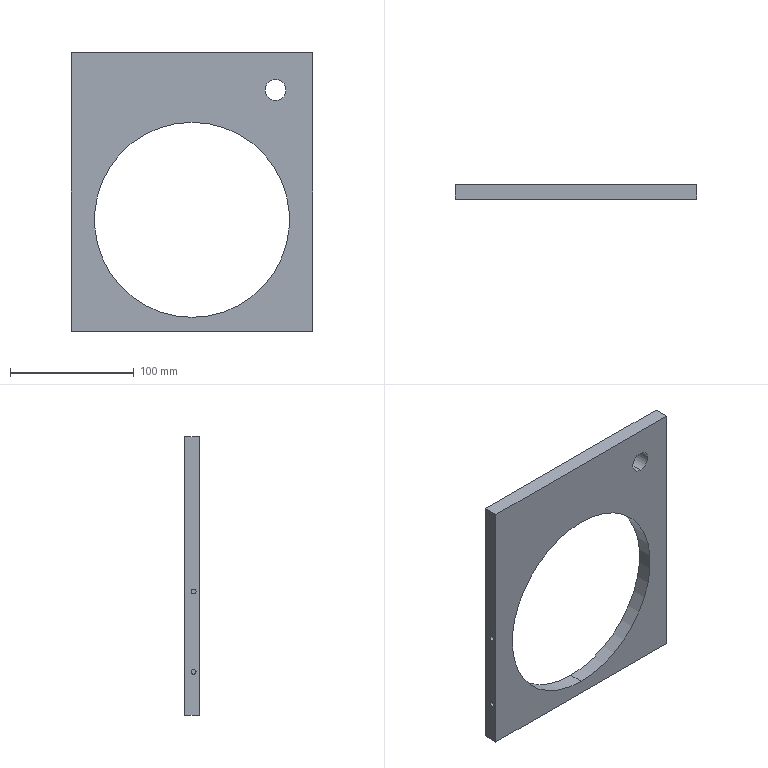Part | STEP file | 2026.6.15-Main Assembly图.sldasm-Part-103 | 1 solid | 40 faces | box 195 x 12 x 225 mm | volume 287509 mm3 | cylinder 24 | plane 16 | commonest cylinder face diameters 6 x16 4 x4 16.875 x2 157.5 x2
STEP:
#1=CARTESIAN_POINT('',(-1676.724,602.301,4218.667));
#2=VERTEX_POINT('',#1);
#3=CARTESIAN_POINT('',(-1676.724,606.301,4218.667));
#4=VERTEX_POINT('',#3);
#5=CARTESIAN_POINT('',(-1676.724,604.301,4218.667));
#6=DIRECTION('',(1.,0.,0.));
#7=DIRECTION('',(0.,-1.,0.));
#8=AXIS2_PLACEMENT_3D('',#5,#6,#7);
#9=CIRCLE('',#8,2.);
#10=EDGE_CURVE('',#2,#4,#9,.T.);
#11=ORIENTED_EDGE('',*,*,#10,.T.);
#12=CARTESIAN_POINT('',(-1686.724,606.301,4218.667));
#13=VERTEX_POINT('',#12);
#14=CARTESIAN_POINT('',(-1676.724,606.301,4218.667));
#15=DIRECTION('',(-1.,0.,0.));
#16=VECTOR('',#15,1000.);
#17=LINE('',#14,#16);
#18=EDGE_CURVE('',#4,#13,#17,.T.);
#19=ORIENTED_EDGE('',*,*,#18,.T.);
#20=CARTESIAN_POINT('',(-1686.724,602.301,4218.667));
#21=VERTEX_POINT('',#20);
#22=CARTESIAN_POINT('',(-1686.724,604.301,4218.667));
#23=DIRECTION('',(-1.,0.,0.));
#24=DIRECTION('',(0.,-1.,0.));
#25=AXIS2_PLACEMENT_3D('',#22,#23,#24);
#26=CIRCLE('',#25,2.);
#27=EDGE_CURVE('',#13,#21,#26,.T.);
#28=ORIENTED_EDGE('',*,*,#27,.T.);
#29=CARTESIAN_POINT('',(-1676.724,602.301,4218.667));
#30=DIRECTION('',(-1.,0.,0.));
#31=VECTOR('',#30,1000.);
#32=LINE('',#29,#31);
#33=EDGE_CURVE('',#2,#21,#32,.T.);
#34=ORIENTED_EDGE('',*,*,#33,.F.);
#35=EDGE_LOOP('',(#11,#19,#28,#34));
#36=FACE_OUTER_BOUND('',#35,.T.);
#37=CARTESIAN_POINT('',(-1676.724,604.301,4218.667));
#38=DIRECTION('',(-1.,0.,0.));
#39=DIRECTION('',(0.,-1.,0.));
#40=AXIS2_PLACEMENT_3D('',#37,#38,#39);
#41=CYLINDRICAL_SURFACE('',#40,2.);
#42=ADVANCED_FACE('',(#36),#41,.F.);
#43=CARTESIAN_POINT('',(-1676.724,602.301,4153.667));
#44=VERTEX_POINT('',#43);
#45=CARTESIAN_POINT('',(-1676.724,606.301,4153.667));
#46=VERTEX_POINT('',#45);
#47=CARTESIAN_POINT('',(-1676.724,604.301,4153.667));
#48=DIRECTION('',(1.,0.,0.));
#49=DIRECTION('',(0.,-1.,0.));
#50=AXIS2_PLACEMENT_3D('',#47,#48,#49);
#51=CIRCLE('',#50,2.);
#52=EDGE_CURVE('',#44,#46,#51,.T.);
#53=ORIENTED_EDGE('',*,*,#52,.T.);
#54=CARTESIAN_POINT('',(-1686.724,606.301,4153.667));
#55=VERTEX_POINT('',#54);
#56=CARTESIAN_POINT('',(-1676.724,606.301,4153.667));
#57=DIRECTION('',(-1.,0.,0.));
#58=VECTOR('',#57,1000.);
#59=LINE('',#56,#58);
#60=EDGE_CURVE('',#46,#55,#59,.T.);
#61=ORIENTED_EDGE('',*,*,#60,.T.);
#62=CARTESIAN_POINT('',(-1686.724,602.301,4153.667));
#63=VERTEX_POINT('',#62);
#64=CARTESIAN_POINT('',(-1686.724,604.301,4153.667));
#65=DIRECTION('',(-1.,0.,0.));
#66=DIRECTION('',(0.,-1.,0.));
#67=AXIS2_PLACEMENT_3D('',#64,#65,#66);
#68=CIRCLE('',#67,2.);
#69=EDGE_CURVE('',#55,#63,#68,.T.);
#70=ORIENTED_EDGE('',*,*,#69,.T.);
#71=CARTESIAN_POINT('',(-1676.724,602.301,4153.667));
#72=DIRECTION('',(-1.,0.,0.));
#73=VECTOR('',#72,1000.);
#74=LINE('',#71,#73);
#75=EDGE_CURVE('',#44,#63,#74,.T.);
#76=ORIENTED_EDGE('',*,*,#75,.F.);
#77=EDGE_LOOP('',(#53,#61,#70,#76));
#78=FACE_OUTER_BOUND('',#77,.T.);
#79=CARTESIAN_POINT('',(-1676.724,604.301,4153.667));
#80=DIRECTION('',(-1.,0.,0.));
#81=DIRECTION('',(0.,-1.,0.));
#82=AXIS2_PLACEMENT_3D('',#79,#80,#81);
#83=CYLINDRICAL_SURFACE('',#82,2.);
#84=ADVANCED_FACE('',(#78),#83,.F.);
#85=CARTESIAN_POINT('',(-1631.724,601.551,4125.667));
#86=VERTEX_POINT('',#85);
#87=CARTESIAN_POINT('',(-1631.724,601.551,4131.667));
#88=VERTEX_POINT('',#87);
#89=CARTESIAN_POINT('',(-1631.724,601.551,4128.667));
#90=DIRECTION('',(0.,1.,0.));
#91=DIRECTION('',(0.,0.,1.));
#92=AXIS2_PLACEMENT_3D('',#89,#90,#91);
#93=CIRCLE('',#92,3.);
#94=EDGE_CURVE('',#86,#88,#93,.T.);
#95=ORIENTED_EDGE('',*,*,#94,.F.);
#96=CARTESIAN_POINT('',(-1631.724,611.551,4125.667));
#97=VERTEX_POINT('',#96);
#98=CARTESIAN_POINT('',(-1631.724,601.551,4125.667));
#99=DIRECTION('',(0.,1.,0.));
#100=VECTOR('',#99,1000.);
#101=LINE('',#98,#100);
#102=EDGE_CURVE('',#86,#97,#101,.T.);
#103=ORIENTED_EDGE('',*,*,#102,.T.);
#104=CARTESIAN_POINT('',(-1631.724,611.551,4131.667));
#105=VERTEX_POINT('',#104);
#106=CARTESIAN_POINT('',(-1631.724,611.551,4128.667));
#107=DIRECTION('',(0.,-1.,0.));
#108=DIRECTION('',(0.,0.,1.));
#109=AXIS2_PLACEMENT_3D('',#106,#107,#108);
#110=CIRCLE('',#109,3.);
#111=EDGE_CURVE('',#105,#97,#110,.T.);
#112=ORIENTED_EDGE('',*,*,#111,.F.);
#113=CARTESIAN_POINT('',(-1631.724,601.551,4131.667));
#114=DIRECTION('',(0.,1.,0.));
#115=VECTOR('',#114,1000.);
#116=LINE('',#113,#115);
#117=EDGE_CURVE('',#88,#105,#116,.T.);
#118=ORIENTED_EDGE('',*,*,#117,.F.);
#119=EDGE_LOOP('',(#95,#103,#112,#118));
#120=FACE_OUTER_BOUND('',#119,.T.);
#121=CARTESIAN_POINT('',(-1631.724,601.551,4128.667));
#122=DIRECTION('',(0.,1.,0.));
#123=DIRECTION('',(0.,0.,1.));
#124=AXIS2_PLACEMENT_3D('',#121,#122,#123);
#125=CYLINDRICAL_SURFACE('',#124,3.);
#126=ADVANCED_FACE('',(#120),#125,.F.);
#127=CARTESIAN_POINT('',(-1546.724,601.551,4131.667));
#128=VERTEX_POINT('',#127);
#129=CARTESIAN_POINT('',(-1546.724,601.551,4125.667));
#130=VERTEX_POINT('',#129);
#131=CARTESIAN_POINT('',(-1546.724,601.551,4128.667));
#132=DIRECTION('',(0.,-1.,0.));
#133=DIRECTION('',(0.,0.,1.));
#134=AXIS2_PLACEMENT_3D('',#131,#132,#133);
#135=CIRCLE('',#134,3.);
#136=EDGE_CURVE('',#128,#130,#135,.T.);
#137=ORIENTED_EDGE('',*,*,#136,.T.);
#138=CARTESIAN_POINT('',(-1546.724,611.551,4125.667));
#139=VERTEX_POINT('',#138);
#140=CARTESIAN_POINT('',(-1546.724,601.551,4125.667));
#141=DIRECTION('',(0.,1.,0.));
#142=VECTOR('',#141,1000.);
#143=LINE('',#140,#142);
#144=EDGE_CURVE('',#130,#139,#143,.T.);
#145=ORIENTED_EDGE('',*,*,#144,.T.);
#146=CARTESIAN_POINT('',(-1546.724,611.551,4131.667));
#147=VERTEX_POINT('',#146);
#148=CARTESIAN_POINT('',(-1546.724,611.551,4128.667));
#149=DIRECTION('',(0.,1.,0.));
#150=DIRECTION('',(0.,0.,1.));
#151=AXIS2_PLACEMENT_3D('',#148,#149,#150);
#152=CIRCLE('',#151,3.);
#153=EDGE_CURVE('',#139,#147,#152,.T.);
#154=ORIENTED_EDGE('',*,*,#153,.T.);
#155=CARTESIAN_POINT('',(-1546.724,601.551,4131.667));
#156=DIRECTION('',(0.,1.,0.));
#157=VECTOR('',#156,1000.);
#158=LINE('',#155,#157);
#159=EDGE_CURVE('',#128,#147,#158,.T.);
#160=ORIENTED_EDGE('',*,*,#159,.F.);
#161=EDGE_LOOP('',(#137,#145,#154,#160));
#162=FACE_OUTER_BOUND('',#161,.T.);
#163=CARTESIAN_POINT('',(-1546.724,601.551,4128.667));
#164=DIRECTION('',(0.,1.,0.));
#165=DIRECTION('',(0.,0.,1.));
#166=AXIS2_PLACEMENT_3D('',#163,#164,#165);
#167=CYLINDRICAL_SURFACE('',#166,3.);
#168=ADVANCED_FACE('',(#162),#167,.F.);
#169=CARTESIAN_POINT('',(-1676.724,601.551,4176.667));
#170=VERTEX_POINT('',#169);
#171=CARTESIAN_POINT('',(-1676.724,601.551,4170.667));
#172=VERTEX_POINT('',#171);
#173=CARTESIAN_POINT('',(-1676.724,601.551,4173.667));
#174=DIRECTION('',(0.,-1.,0.));
#175=DIRECTION('',(0.,0.,1.));
#176=AXIS2_PLACEMENT_3D('',#173,#174,#175);
#177=CIRCLE('',#176,3.);
#178=EDGE_CURVE('',#170,#172,#177,.T.);
#179=ORIENTED_EDGE('',*,*,#178,.T.);
#180=CARTESIAN_POINT('',(-1676.724,611.551,4170.667));
#181=VERTEX_POINT('',#180);
#182=CARTESIAN_POINT('',(-1676.724,601.551,4170.667));
#183=DIRECTION('',(0.,1.,0.));
#184=VECTOR('',#183,1000.);
#185=LINE('',#182,#184);
#186=EDGE_CURVE('',#172,#181,#185,.T.);
#187=ORIENTED_EDGE('',*,*,#186,.T.);
#188=CARTESIAN_POINT('',(-1676.724,611.551,4176.667));
#189=VERTEX_POINT('',#188);
#190=CARTESIAN_POINT('',(-1676.724,611.551,4173.667));
#191=DIRECTION('',(0.,1.,0.));
#192=DIRECTION('',(0.,0.,1.));
#193=AXIS2_PLACEMENT_3D('',#190,#191,#192);
#194=CIRCLE('',#193,3.);
#195=EDGE_CURVE('',#181,#189,#194,.T.);
#196=ORIENTED_EDGE('',*,*,#195,.T.);
#197=CARTESIAN_POINT('',(-1676.724,601.551,4176.667));
#198=DIRECTION('',(0.,1.,0.));
#199=VECTOR('',#198,1000.);
#200=LINE('',#197,#199);
#201=EDGE_CURVE('',#170,#189,#200,.T.);
#202=ORIENTED_EDGE('',*,*,#201,.F.);
#203=EDGE_LOOP('',(#179,#187,#196,#202));
#204=FACE_OUTER_BOUND('',#203,.T.);
#205=CARTESIAN_POINT('',(-1676.724,601.551,4173.667));
#206=DIRECTION('',(0.,1.,0.));
#207=DIRECTION('',(0.,0.,1.));
#208=AXIS2_PLACEMENT_3D('',#205,#206,#207);
#209=CYLINDRICAL_SURFACE('',#208,3.);
#210=ADVANCED_FACE('',(#204),#209,.F.);
#211=CARTESIAN_POINT('',(-1501.724,601.551,4176.667));
#212=VERTEX_POINT('',#211);
#213=CARTESIAN_POINT('',(-1501.724,601.551,4170.667));
#214=VERTEX_POINT('',#213);
#215=CARTESIAN_POINT('',(-1501.724,601.551,4173.667));
#216=DIRECTION('',(0.,-1.,0.));
#217=DIRECTION('',(0.,0.,1.));
#218=AXIS2_PLACEMENT_3D('',#215,#216,#217);
#219=CIRCLE('',#218,3.);
#220=EDGE_CURVE('',#212,#214,#219,.T.);
#221=ORIENTED_EDGE('',*,*,#220,.T.);
#222=CARTESIAN_POINT('',(-1501.724,611.551,4170.667));
#223=VERTEX_POINT('',#222);
#224=CARTESIAN_POINT('',(-1501.724,601.551,4170.667));
#225=DIRECTION('',(0.,1.,0.));
#226=VECTOR('',#225,1000.);
#227=LINE('',#224,#226);
#228=EDGE_CURVE('',#214,#223,#227,.T.);
#229=ORIENTED_EDGE('',*,*,#228,.T.);
#230=CARTESIAN_POINT('',(-1501.724,611.551,4176.667));
#231=VERTEX_POINT('',#230);
#232=CARTESIAN_POINT('',(-1501.724,611.551,4173.667));
#233=DIRECTION('',(0.,1.,0.));
#234=DIRECTION('',(0.,0.,1.));
#235=AXIS2_PLACEMENT_3D('',#232,#233,#234);
#236=CIRCLE('',#235,3.);
#237=EDGE_CURVE('',#223,#231,#236,.T.);
#238=ORIENTED_EDGE('',*,*,#237,.T.);
#239=CARTESIAN_POINT('',(-1501.724,601.551,4176.667));
#240=DIRECTION('',(0.,1.,0.));
#241=VECTOR('',#240,1000.);
#242=LINE('',#239,#241);
#243=EDGE_CURVE('',#212,#231,#242,.T.);
#244=ORIENTED_EDGE('',*,*,#243,.F.);
#245=EDGE_LOOP('',(#221,#229,#238,#244));
#246=FACE_OUTER_BOUND('',#245,.T.);
#247=CARTESIAN_POINT('',(-1501.724,601.551,4173.667));
#248=DIRECTION('',(0.,1.,0.));
#249=DIRECTION('',(0.,0.,1.));
#250=AXIS2_PLACEMENT_3D('',#247,#248,#249);
#251=CYLINDRICAL_SURFACE('',#250,3.);
#252=ADVANCED_FACE('',(#246),#251,.F.);
#253=CARTESIAN_POINT('',(-1676.724,601.551,4246.667));
#254=VERTEX_POINT('',#253);
#255=CARTESIAN_POINT('',(-1676.724,601.551,4240.667));
#256=VERTEX_POINT('',#255);
#257=CARTESIAN_POINT('',(-1676.724,601.551,4243.667));
#258=DIRECTION('',(0.,-1.,0.));
#259=DIRECTION('',(0.,0.,1.));
#260=AXIS2_PLACEMENT_3D('',#257,#258,#259);
#261=CIRCLE('',#260,3.);
#262=EDGE_CURVE('',#254,#256,#261,.T.);
#263=ORIENTED_EDGE('',*,*,#262,.T.);
#264=CARTESIAN_POINT('',(-1676.724,611.551,4240.667));
#265=VERTEX_POINT('',#264);
#266=CARTESIAN_POINT('',(-1676.724,601.551,4240.667));
#267=DIRECTION('',(0.,1.,0.));
#268=VECTOR('',#267,1000.);
#269=LINE('',#266,#268);
#270=EDGE_CURVE('',#256,#265,#269,.T.);
#271=ORIENTED_EDGE('',*,*,#270,.T.);
#272=CARTESIAN_POINT('',(-1676.724,611.551,4246.667));
#273=VERTEX_POINT('',#272);
#274=CARTESIAN_POINT('',(-1676.724,611.551,4243.667));
#275=DIRECTION('',(0.,1.,0.));
#276=DIRECTION('',(0.,0.,1.));
#277=AXIS2_PLACEMENT_3D('',#274,#275,#276);
#278=CIRCLE('',#277,3.);
#279=EDGE_CURVE('',#265,#273,#278,.T.);
#280=ORIENTED_EDGE('',*,*,#279,.T.);
#281=CARTESIAN_POINT('',(-1676.724,601.551,4246.667));
#282=DIRECTION('',(0.,1.,0.));
#283=VECTOR('',#282,1000.);
#284=LINE('',#281,#283);
#285=EDGE_CURVE('',#254,#273,#284,.T.);
#286=ORIENTED_EDGE('',*,*,#285,.F.);
#287=EDGE_LOOP('',(#263,#271,#280,#286));
#288=FACE_OUTER_BOUND('',#287,.T.);
#289=CARTESIAN_POINT('',(-1676.724,601.551,4243.667));
#290=DIRECTION('',(0.,1.,0.));
#291=DIRECTION('',(0.,0.,1.));
#292=AXIS2_PLACEMENT_3D('',#289,#290,#291);
#293=CYLINDRICAL_SURFACE('',#292,3.);
#294=ADVANCED_FACE('',(#288),#293,.F.);
#295=CARTESIAN_POINT('',(-1501.724,601.551,4246.667));
#296=VERTEX_POINT('',#295);
#297=CARTESIAN_POINT('',(-1501.724,601.551,4240.667));
#298=VERTEX_POINT('',#297);
#299=CARTESIAN_POINT('',(-1501.724,601.551,4243.667));
#300=DIRECTION('',(0.,-1.,0.));
#301=DIRECTION('',(0.,0.,1.));
#302=AXIS2_PLACEMENT_3D('',#299,#300,#301);
#303=CIRCLE('',#302,3.);
#304=EDGE_CURVE('',#296,#298,#303,.T.);
#305=ORIENTED_EDGE('',*,*,#304,.T.);
#306=CARTESIAN_POINT('',(-1501.724,611.551,4240.667));
#307=VERTEX_POINT('',#306);
#308=CARTESIAN_POINT('',(-1501.724,601.551,4240.667));
#309=DIRECTION('',(0.,1.,0.));
#310=VECTOR('',#309,1000.);
#311=LINE('',#308,#310);
#312=EDGE_CURVE('',#298,#307,#311,.T.);
#313=ORIENTED_EDGE('',*,*,#312,.T.);
#314=CARTESIAN_POINT('',(-1501.724,611.551,4246.667));
#315=VERTEX_POINT('',#314);
#316=CARTESIAN_POINT('',(-1501.724,611.551,4243.667));
#317=DIRECTION('',(0.,1.,0.));
#318=DIRECTION('',(0.,0.,1.));
#319=AXIS2_PLACEMENT_3D('',#316,#317,#318);
#320=CIRCLE('',#319,3.);
#321=EDGE_CURVE('',#307,#315,#320,.T.);
#322=ORIENTED_EDGE('',*,*,#321,.T.);
#323=CARTESIAN_POINT('',(-1501.724,601.551,4246.667));
#324=DIRECTION('',(0.,1.,0.));
#325=VECTOR('',#324,1000.);
#326=LINE('',#323,#325);
#327=EDGE_CURVE('',#296,#315,#326,.T.);
#328=ORIENTED_EDGE('',*,*,#327,.F.);
#329=EDGE_LOOP('',(#305,#313,#322,#328));
#330=FACE_OUTER_BOUND('',#329,.T.);
#331=CARTESIAN_POINT('',(-1501.724,601.551,4243.667));
#332=DIRECTION('',(0.,1.,0.));
#333=DIRECTION('',(0.,0.,1.));
#334=AXIS2_PLACEMENT_3D('',#331,#332,#333);
#335=CYLINDRICAL_SURFACE('',#334,3.);
#336=ADVANCED_FACE('',(#330),#335,.F.);
#337=CARTESIAN_POINT('',(-1631.724,601.551,4291.667));
#338=VERTEX_POINT('',#337);
#339=CARTESIAN_POINT('',(-1631.724,601.551,4285.667));
#340=VERTEX_POINT('',#339);
#341=CARTESIAN_POINT('',(-1631.724,601.551,4288.667));
#342=DIRECTION('',(0.,-1.,0.));
#343=DIRECTION('',(0.,0.,1.));
#344=AXIS2_PLACEMENT_3D('',#341,#342,#343);
#345=CIRCLE('',#344,3.);
#346=EDGE_CURVE('',#338,#340,#345,.T.);
#347=ORIENTED_EDGE('',*,*,#346,.T.);
#348=CARTESIAN_POINT('',(-1631.724,611.551,4285.667));
#349=VERTEX_POINT('',#348);
#350=CARTESIAN_POINT('',(-1631.724,601.551,4285.667));
#351=DIRECTION('',(0.,1.,0.));
#352=VECTOR('',#351,1000.);
#353=LINE('',#350,#352);
#354=EDGE_CURVE('',#340,#349,#353,.T.);
#355=ORIENTED_EDGE('',*,*,#354,.T.);
#356=CARTESIAN_POINT('',(-1631.724,611.551,4291.667));
#357=VERTEX_POINT('',#356);
#358=CARTESIAN_POINT('',(-1631.724,611.551,4288.667));
#359=DIRECTION('',(0.,1.,0.));
#360=DIRECTION('',(0.,0.,1.));
#361=AXIS2_PLACEMENT_3D('',#358,#359,#360);
#362=CIRCLE('',#361,3.);
#363=EDGE_CURVE('',#349,#357,#362,.T.);
#364=ORIENTED_EDGE('',*,*,#363,.T.);
#365=CARTESIAN_POINT('',(-1631.724,601.551,4291.667));
#366=DIRECTION('',(0.,1.,0.));
#367=VECTOR('',#366,1000.);
#368=LINE('',#365,#367);
#369=EDGE_CURVE('',#338,#357,#368,.T.);
#370=ORIENTED_EDGE('',*,*,#369,.F.);
#371=EDGE_LOOP('',(#347,#355,#364,#370));
#372=FACE_OUTER_BOUND('',#371,.T.);
#373=CARTESIAN_POINT('',(-1631.724,601.551,4288.667));
#374=DIRECTION('',(0.,1.,0.));
#375=DIRECTION('',(0.,0.,1.));
#376=AXIS2_PLACEMENT_3D('',#373,#374,#375);
#377=CYLINDRICAL_SURFACE('',#376,3.);
#378=ADVANCED_FACE('',(#372),#377,.F.);
#379=CARTESIAN_POINT('',(-1546.724,601.551,4291.667));
#380=VERTEX_POINT('',#379);
#381=CARTESIAN_POINT('',(-1546.724,601.551,4285.667));
#382=VERTEX_POINT('',#381);
#383=CARTESIAN_POINT('',(-1546.724,601.551,4288.667));
#384=DIRECTION('',(0.,-1.,0.));
#385=DIRECTION('',(0.,0.,1.));
#386=AXIS2_PLACEMENT_3D('',#383,#384,#385);
#387=CIRCLE('',#386,3.);
#388=EDGE_CURVE('',#380,#382,#387,.T.);
#389=ORIENTED_EDGE('',*,*,#388,.T.);
#390=CARTESIAN_POINT('',(-1546.724,611.551,4285.667));
#391=VERTEX_POINT('',#390);
#392=CARTESIAN_POINT('',(-1546.724,601.551,4285.667));
#393=DIRECTION('',(0.,1.,0.));
#394=VECTOR('',#393,1000.);
#395=LINE('',#392,#394);
#396=EDGE_CURVE('',#382,#391,#395,.T.);
#397=ORIENTED_EDGE('',*,*,#396,.T.);
#398=CARTESIAN_POINT('',(-1546.724,611.551,4291.667));
#399=VERTEX_POINT('',#398);
#400=CARTESIAN_POINT('',(-1546.724,611.551,4288.667));
#401=DIRECTION('',(0.,1.,0.));
#402=DIRECTION('',(0.,0.,1.));
#403=AXIS2_PLACEMENT_3D('',#400,#401,#402);
#404=CIRCLE('',#403,3.);
#405=EDGE_CURVE('',#391,#399,#404,.T.);
#406=ORIENTED_EDGE('',*,*,#405,.T.);
#407=CARTESIAN_POINT('',(-1546.724,601.551,4291.667));
#408=DIRECTION('',(0.,1.,0.));
#409=VECTOR('',#408,1000.);
#410=LINE('',#407,#409);
#411=EDGE_CURVE('',#380,#399,#410,.T.);
#412=ORIENTED_EDGE('',*,*,#411,.F.);
#413=EDGE_LOOP('',(#389,#397,#406,#412));
#414=FACE_OUTER_BOUND('',#413,.T.);
#415=CARTESIAN_POINT('',(-1546.724,601.551,4288.667));
#416=DIRECTION('',(0.,1.,0.));
#417=DIRECTION('',(0.,0.,1.));
#418=AXIS2_PLACEMENT_3D('',#415,#416,#417);
#419=CYLINDRICAL_SURFACE('',#418,3.);
#420=ADVANCED_FACE('',(#414),#419,.F.);
#421=CARTESIAN_POINT('',(-1589.224,599.551,4129.917));
#422=VERTEX_POINT('',#421);
#423=CARTESIAN_POINT('',(-1589.224,599.551,4287.417));
#424=VERTEX_POINT('',#423);
#425=CARTESIAN_POINT('',(-1589.224,599.551,4208.667));
#426=DIRECTION('',(0.,1.,0.));
#427=DIRECTION('',(0.,0.,1.));
#428=AXIS2_PLACEMENT_3D('',#425,#426,#427);
#429=CIRCLE('',#428,78.75);
#430=EDGE_CURVE('',#422,#424,#429,.T.);
#431=ORIENTED_EDGE('',*,*,#430,.F.);
#432=CARTESIAN_POINT('',(-1589.224,611.551,4129.917));
#433=VERTEX_POINT('',#432);
#434=CARTESIAN_POINT('',(-1589.224,599.551,4129.917));
#435=DIRECTION('',(0.,1.,0.));
#436=VECTOR('',#435,1000.);
#437=LINE('',#434,#436);
#438=EDGE_CURVE('',#422,#433,#437,.T.);
#439=ORIENTED_EDGE('',*,*,#438,.T.);
#440=CARTESIAN_POINT('',(-1589.224,611.551,4287.417));
#441=VERTEX_POINT('',#440);
#442=CARTESIAN_POINT('',(-1589.224,611.551,4208.667));
#443=DIRECTION('',(0.,1.,0.));
#444=DIRECTION('',(0.,0.,1.));
#445=AXIS2_PLACEMENT_3D('',#442,#443,#444);
#446=CIRCLE('',#445,78.75);
#447=EDGE_CURVE('',#433,#441,#446,.T.);
#448=ORIENTED_EDGE('',*,*,#447,.T.);
#449=CARTESIAN_POINT('',(-1589.224,599.551,4287.417));
#450=DIRECTION('',(0.,1.,0.));
#451=VECTOR('',#450,1000.);
#452=LINE('',#449,#451);
#453=EDGE_CURVE('',#424,#441,#452,.T.);
#454=ORIENTED_EDGE('',*,*,#453,.F.);
#455=EDGE_LOOP('',(#431,#439,#448,#454));
#456=FACE_OUTER_BOUND('',#455,.T.);
#457=CARTESIAN_POINT('',(-1589.224,599.551,4208.667));
#458=DIRECTION('',(0.,1.,0.));
#459=DIRECTION('',(0.,0.,1.));
#460=AXIS2_PLACEMENT_3D('',#457,#458,#459);
#461=CYLINDRICAL_SURFACE('',#460,78.75);
#462=ADVANCED_FACE('',(#456),#461,.F.);
#463=CARTESIAN_POINT('',(-1521.724,599.551,4305.229));
#464=VERTEX_POINT('',#463);
#465=CARTESIAN_POINT('',(-1521.724,599.551,4322.104));
#466=VERTEX_POINT('',#465);
#467=CARTESIAN_POINT('',(-1521.724,599.551,4313.667));
#468=DIRECTION('',(0.,1.,0.));
#469=DIRECTION('',(0.,0.,1.));
#470=AXIS2_PLACEMENT_3D('',#467,#468,#469);
#471=CIRCLE('',#470,8.438);
#472=EDGE_CURVE('',#464,#466,#471,.T.);
#473=ORIENTED_EDGE('',*,*,#472,.F.);
#474=CARTESIAN_POINT('',(-1521.724,611.551,4305.229));
#475=VERTEX_POINT('',#474);
#476=CARTESIAN_POINT('',(-1521.724,599.551,4305.229));
#477=DIRECTION('',(0.,1.,0.));
#478=VECTOR('',#477,1000.);
#479=LINE('',#476,#478);
#480=EDGE_CURVE('',#464,#475,#479,.T.);
#481=ORIENTED_EDGE('',*,*,#480,.T.);
#482=CARTESIAN_POINT('',(-1521.724,611.551,4322.104));
#483=VERTEX_POINT('',#482);
#484=CARTESIAN_POINT('',(-1521.724,611.551,4313.667));
#485=DIRECTION('',(0.,1.,0.));
#486=DIRECTION('',(0.,0.,1.));
#487=AXIS2_PLACEMENT_3D('',#484,#485,#486);
#488=CIRCLE('',#487,8.438);
#489=EDGE_CURVE('',#475,#483,#488,.T.);
#490=ORIENTED_EDGE('',*,*,#489,.T.);
#491=CARTESIAN_POINT('',(-1521.724,599.551,4322.104));
#492=DIRECTION('',(0.,1.,0.));
#493=VECTOR('',#492,1000.);
#494=LINE('',#491,#493);
#495=EDGE_CURVE('',#466,#483,#494,.T.);
#496=ORIENTED_EDGE('',*,*,#495,.F.);
#497=EDGE_LOOP('',(#473,#481,#490,#496));
#498=FACE_OUTER_BOUND('',#497,.T.);
#499=CARTESIAN_POINT('',(-1521.724,599.551,4313.667));
#500=DIRECTION('',(0.,1.,0.));
#501=DIRECTION('',(0.,0.,1.));
#502=AXIS2_PLACEMENT_3D('',#499,#500,#501);
#503=CYLINDRICAL_SURFACE('',#502,8.438);
#504=ADVANCED_FACE('',(#498),#503,.F.);
#505=CARTESIAN_POINT('',(-1491.724,611.551,4118.667));
#506=VERTEX_POINT('',#505);
#507=CARTESIAN_POINT('',(-1491.724,611.551,4343.667));
#508=VERTEX_POINT('',#507);
#509=CARTESIAN_POINT('',(-1491.724,611.551,4118.667));
#510=DIRECTION('',(0.,0.,1.));
#511=VECTOR('',#510,1000.);
#512=LINE('',#509,#511);
#513=EDGE_CURVE('',#506,#508,#512,.T.);
#514=ORIENTED_EDGE('',*,*,#513,.T.);
#515=CARTESIAN_POINT('',(-1491.724,599.551,4343.667));
#516=VERTEX_POINT('',#515);
#517=CARTESIAN_POINT('',(-1491.724,599.551,4343.667));
#518=DIRECTION('',(0.,1.,0.));
#519=VECTOR('',#518,1000.);
#520=LINE('',#517,#519);
#521=EDGE_CURVE('',#516,#508,#520,.T.);
#522=ORIENTED_EDGE('',*,*,#521,.F.);
#523=CARTESIAN_POINT('',(-1491.724,599.551,4118.667));
#524=VERTEX_POINT('',#523);
#525=CARTESIAN_POINT('',(-1491.724,599.551,4118.667));
#526=DIRECTION('',(0.,0.,1.));
#527=VECTOR('',#526,1000.);
#528=LINE('',#525,#527);
#529=EDGE_CURVE('',#524,#516,#528,.T.);
#530=ORIENTED_EDGE('',*,*,#529,.F.);
#531=CARTESIAN_POINT('',(-1491.724,599.551,4118.667));
#532=DIRECTION('',(0.,1.,0.));
#533=VECTOR('',#532,1000.);
#534=LINE('',#531,#533);
#535=EDGE_CURVE('',#524,#506,#534,.T.);
#536=ORIENTED_EDGE('',*,*,#535,.T.);
#537=EDGE_LOOP('',(#514,#522,#530,#536));
#538=FACE_OUTER_BOUND('',#537,.T.);
#539=CARTESIAN_POINT('',(-1491.724,599.551,4118.667));
#540=DIRECTION('',(-1.,0.,0.));
#541=DIRECTION('',(0.,-1.,0.));
#542=AXIS2_PLACEMENT_3D('',#539,#540,#541);
#543=PLANE('',#542);
#544=ADVANCED_FACE('',(#538),#543,.F.);
#545=CARTESIAN_POINT('',(-1686.724,611.551,4343.667));
#546=VERTEX_POINT('',#545);
#547=CARTESIAN_POINT('',(-1491.724,611.551,4343.667));
#548=DIRECTION('',(-1.,0.,0.));
#549=VECTOR('',#548,1000.);
#550=LINE('',#547,#549);
#551=EDGE_CURVE('',#508,#546,#550,.T.);
#552=ORIENTED_EDGE('',*,*,#551,.T.);
#553=CARTESIAN_POINT('',(-1686.724,599.551,4343.667));
#554=VERTEX_POINT('',#553);
#555=CARTESIAN_POINT('',(-1686.724,599.551,4343.667));
#556=DIRECTION('',(0.,1.,0.));
#557=VECTOR('',#556,1000.);
#558=LINE('',#555,#557);
#559=EDGE_CURVE('',#554,#546,#558,.T.);
#560=ORIENTED_EDGE('',*,*,#559,.F.);
#561=CARTESIAN_POINT('',(-1491.724,599.551,4343.667));
#562=DIRECTION('',(-1.,0.,0.));
#563=VECTOR('',#562,1000.);
#564=LINE('',#561,#563);
#565=EDGE_CURVE('',#516,#554,#564,.T.);
#566=ORIENTED_EDGE('',*,*,#565,.F.);
#567=ORIENTED_EDGE('',*,*,#521,.T.);
#568=EDGE_LOOP('',(#552,#560,#566,#567));
#569=FACE_OUTER_BOUND('',#568,.T.);
#570=CARTESIAN_POINT('',(-1491.724,599.551,4343.667));
#571=DIRECTION('',(0.,0.,-1.));
#572=DIRECTION('',(-1.,0.,0.));
#573=AXIS2_PLACEMENT_3D('',#570,#571,#572);
#574=PLANE('',#573);
#575=ADVANCED_FACE('',(#569),#574,.F.);
#576=CARTESIAN_POINT('',(-1686.724,604.301,4218.667));
#577=DIRECTION('',(-1.,0.,0.));
#578=DIRECTION('',(0.,-1.,0.));
#579=AXIS2_PLACEMENT_3D('',#576,#577,#578);
#580=CIRCLE('',#579,2.);
#581=EDGE_CURVE('',#21,#13,#580,.T.);
#582=ORIENTED_EDGE('',*,*,#581,.F.);
#583=ORIENTED_EDGE('',*,*,#27,.F.);
#584=EDGE_LOOP('',(#582,#583));
#585=FACE_BOUND('',#584,.T.);
#586=CARTESIAN_POINT('',(-1686.724,604.301,4153.667));
#587=DIRECTION('',(-1.,0.,0.));
#588=DIRECTION('',(0.,-1.,0.));
#589=AXIS2_PLACEMENT_3D('',#586,#587,#588);
#590=CIRCLE('',#589,2.);
#591=EDGE_CURVE('',#63,#55,#590,.T.);
#592=ORIENTED_EDGE('',*,*,#591,.F.);
#593=ORIENTED_EDGE('',*,*,#69,.F.);
#594=EDGE_LOOP('',(#592,#593));
#595=FACE_BOUND('',#594,.T.);
#596=CARTESIAN_POINT('',(-1686.724,611.551,4118.667));
#597=VERTEX_POINT('',#596);
#598=CARTESIAN_POINT('',(-1686.724,611.551,4343.667));
#599=DIRECTION('',(0.,0.,-1.));
#600=VECTOR('',#599,1000.);
#601=LINE('',#598,#600);
#602=EDGE_CURVE('',#546,#597,#601,.T.);
#603=ORIENTED_EDGE('',*,*,#602,.T.);
#604=CARTESIAN_POINT('',(-1686.724,599.551,4118.667));
#605=VERTEX_POINT('',#604);
#606=CARTESIAN_POINT('',(-1686.724,599.551,4118.667));
#607=DIRECTION('',(0.,1.,0.));
#608=VECTOR('',#607,1000.);
#609=LINE('',#606,#608);
#610=EDGE_CURVE('',#605,#597,#609,.T.);
#611=ORIENTED_EDGE('',*,*,#610,.F.);
#612=CARTESIAN_POINT('',(-1686.724,599.551,4343.667));
#613=DIRECTION('',(0.,0.,-1.));
#614=VECTOR('',#613,1000.);
#615=LINE('',#612,#614);
#616=EDGE_CURVE('',#554,#605,#615,.T.);
#617=ORIENTED_EDGE('',*,*,#616,.F.);
#618=ORIENTED_EDGE('',*,*,#559,.T.);
#619=EDGE_LOOP('',(#603,#611,#617,#618));
#620=FACE_OUTER_BOUND('',#619,.T.);
#621=CARTESIAN_POINT('',(-1686.724,599.551,4343.667));
#622=DIRECTION('',(1.,0.,0.));
#623=DIRECTION('',(0.,1.,0.));
#624=AXIS2_PLACEMENT_3D('',#621,#622,#623);
#625=PLANE('',#624);
#626=ADVANCED_FACE('',(#585,#595,#620),#625,.F.);
#627=ORIENTED_EDGE('',*,*,#480,.F.);
#628=CARTESIAN_POINT('',(-1521.724,599.551,4313.667));
#629=DIRECTION('',(0.,1.,0.));
#630=DIRECTION('',(0.,0.,1.));
#631=AXIS2_PLACEMENT_3D('',#628,#629,#630);
#632=CIRCLE('',#631,8.438);
#633=EDGE_CURVE('',#466,#464,#632,.T.);
#634=ORIENTED_EDGE('',*,*,#633,.F.);
#635=ORIENTED_EDGE('',*,*,#495,.T.);
#636=CARTESIAN_POINT('',(-1521.724,611.551,4313.667));
#637=DIRECTION('',(0.,1.,0.));
#638=DIRECTION('',(0.,0.,1.));
#639=AXIS2_PLACEMENT_3D('',#636,#637,#638);
#640=CIRCLE('',#639,8.438);
#641=EDGE_CURVE('',#483,#475,#640,.T.);
#642=ORIENTED_EDGE('',*,*,#641,.T.);
#643=EDGE_LOOP('',(#627,#634,#635,#642));
#644=FACE_OUTER_BOUND('',#643,.T.);
#645=CARTESIAN_POINT('',(-1521.724,599.551,4313.667));
#646=DIRECTION('',(0.,1.,0.));
#647=DIRECTION('',(0.,0.,1.));
#648=AXIS2_PLACEMENT_3D('',#645,#646,#647);
#649=CYLINDRICAL_SURFACE('',#648,8.438);
#650=ADVANCED_FACE('',(#644),#649,.F.);
#651=CARTESIAN_POINT('',(-1686.724,611.551,4118.667));
#652=DIRECTION('',(1.,0.,0.));
#653=VECTOR('',#652,1000.);
#654=LINE('',#651,#653);
#655=EDGE_CURVE('',#597,#506,#654,.T.);
#656=ORIENTED_EDGE('',*,*,#655,.T.);
#657=ORIENTED_EDGE('',*,*,#535,.F.);
#658=CARTESIAN_POINT('',(-1686.724,599.551,4118.667));
#659=DIRECTION('',(1.,0.,0.));
#660=VECTOR('',#659,1000.);
#661=LINE('',#658,#660);
#662=EDGE_CURVE('',#605,#524,#661,.T.);
#663=ORIENTED_EDGE('',*,*,#662,.F.);
#664=ORIENTED_EDGE('',*,*,#610,.T.);
#665=EDGE_LOOP('',(#656,#657,#663,#664));
#666=FACE_OUTER_BOUND('',#665,.T.);
#667=CARTESIAN_POINT('',(-1686.724,599.551,4118.667));
#668=DIRECTION('',(0.,0.,1.));
#669=DIRECTION('',(1.,0.,0.));
#670=AXIS2_PLACEMENT_3D('',#667,#668,#669);
#671=PLANE('',#670);
#672=ADVANCED_FACE('',(#666),#671,.F.);
#673=ORIENTED_EDGE('',*,*,#438,.F.);
#674=CARTESIAN_POINT('',(-1589.224,599.551,4208.667));
#675=DIRECTION('',(0.,1.,0.));
#676=DIRECTION('',(0.,0.,1.));
#677=AXIS2_PLACEMENT_3D('',#674,#675,#676);
#678=CIRCLE('',#677,78.75);
#679=EDGE_CURVE('',#424,#422,#678,.T.);
#680=ORIENTED_EDGE('',*,*,#679,.F.);
#681=ORIENTED_EDGE('',*,*,#453,.T.);
#682=CARTESIAN_POINT('',(-1589.224,611.551,4208.667));
#683=DIRECTION('',(0.,1.,0.));
#684=DIRECTION('',(0.,0.,1.));
#685=AXIS2_PLACEMENT_3D('',#682,#683,#684);
#686=CIRCLE('',#685,78.75);
#687=EDGE_CURVE('',#441,#433,#686,.T.);
#688=ORIENTED_EDGE('',*,*,#687,.T.);
#689=EDGE_LOOP('',(#673,#680,#681,#688));
#690=FACE_OUTER_BOUND('',#689,.T.);
#691=CARTESIAN_POINT('',(-1589.224,599.551,4208.667));
#692=DIRECTION('',(0.,1.,0.));
#693=DIRECTION('',(0.,0.,1.));
#694=AXIS2_PLACEMENT_3D('',#691,#692,#693);
#695=CYLINDRICAL_SURFACE('',#694,78.75);
#696=ADVANCED_FACE('',(#690),#695,.F.);
#697=ORIENTED_EDGE('',*,*,#529,.T.);
#698=ORIENTED_EDGE('',*,*,#565,.T.);
#699=ORIENTED_EDGE('',*,*,#616,.T.);
#700=ORIENTED_EDGE('',*,*,#662,.T.);
#701=EDGE_LOOP('',(#697,#698,#699,#700));
#702=FACE_OUTER_BOUND('',#701,.T.);
#703=ORIENTED_EDGE('',*,*,#633,.T.);
#704=ORIENTED_EDGE('',*,*,#472,.T.);
#705=EDGE_LOOP('',(#703,#704));
#706=FACE_BOUND('',#705,.T.);
#707=ORIENTED_EDGE('',*,*,#679,.T.);
#708=ORIENTED_EDGE('',*,*,#430,.T.);
#709=EDGE_LOOP('',(#707,#708));
#710=FACE_BOUND('',#709,.T.);
#711=CARTESIAN_POINT('',(-1521.724,599.551,4313.667));
#712=DIRECTION('',(0.,1.,0.));
#713=DIRECTION('',(0.,0.,1.));
#714=AXIS2_PLACEMENT_3D('',#711,#712,#713);
#715=PLANE('',#714);
#716=ADVANCED_FACE('',(#702,#706,#710),#715,.F.);
#717=ORIENTED_EDGE('',*,*,#111,.T.);
#718=CARTESIAN_POINT('',(-1631.724,611.551,4128.667));
#719=DIRECTION('',(0.,-1.,0.));
#720=DIRECTION('',(0.,0.,1.));
#721=AXIS2_PLACEMENT_3D('',#718,#719,#720);
#722=CIRCLE('',#721,3.);
#723=EDGE_CURVE('',#97,#105,#722,.T.);
#724=ORIENTED_EDGE('',*,*,#723,.T.);
#725=EDGE_LOOP('',(#717,#724));
#726=FACE_BOUND('',#725,.T.);
#727=CARTESIAN_POINT('',(-1546.724,611.551,4128.667));
#728=DIRECTION('',(0.,1.,0.));
#729=DIRECTION('',(0.,0.,1.));
#730=AXIS2_PLACEMENT_3D('',#727,#728,#729);
#731=CIRCLE('',#730,3.);
#732=EDGE_CURVE('',#147,#139,#731,.T.);
#733=ORIENTED_EDGE('',*,*,#732,.F.);
#734=ORIENTED_EDGE('',*,*,#153,.F.);
#735=EDGE_LOOP('',(#733,#734));
#736=FACE_BOUND('',#735,.T.);
#737=CARTESIAN_POINT('',(-1676.724,611.551,4173.667));
#738=DIRECTION('',(0.,1.,0.));
#739=DIRECTION('',(0.,0.,1.));
#740=AXIS2_PLACEMENT_3D('',#737,#738,#739);
#741=CIRCLE('',#740,3.);
#742=EDGE_CURVE('',#189,#181,#741,.T.);
#743=ORIENTED_EDGE('',*,*,#742,.F.);
#744=ORIENTED_EDGE('',*,*,#195,.F.);
#745=EDGE_LOOP('',(#743,#744));
#746=FACE_BOUND('',#745,.T.);
#747=CARTESIAN_POINT('',(-1501.724,611.551,4173.667));
#748=DIRECTION('',(0.,1.,0.));
#749=DIRECTION('',(0.,0.,1.));
#750=AXIS2_PLACEMENT_3D('',#747,#748,#749);
#751=CIRCLE('',#750,3.);
#752=EDGE_CURVE('',#231,#223,#751,.T.);
#753=ORIENTED_EDGE('',*,*,#752,.F.);
#754=ORIENTED_EDGE('',*,*,#237,.F.);
#755=EDGE_LOOP('',(#753,#754));
#756=FACE_BOUND('',#755,.T.);
#757=CARTESIAN_POINT('',(-1676.724,611.551,4243.667));
#758=DIRECTION('',(0.,1.,0.));
#759=DIRECTION('',(0.,0.,1.));
#760=AXIS2_PLACEMENT_3D('',#757,#758,#759);
#761=CIRCLE('',#760,3.);
#762=EDGE_CURVE('',#273,#265,#761,.T.);
#763=ORIENTED_EDGE('',*,*,#762,.F.);
#764=ORIENTED_EDGE('',*,*,#279,.F.);
#765=EDGE_LOOP('',(#763,#764));
#766=FACE_BOUND('',#765,.T.);
#767=CARTESIAN_POINT('',(-1501.724,611.551,4243.667));
#768=DIRECTION('',(0.,1.,0.));
#769=DIRECTION('',(0.,0.,1.));
#770=AXIS2_PLACEMENT_3D('',#767,#768,#769);
#771=CIRCLE('',#770,3.);
#772=EDGE_CURVE('',#315,#307,#771,.T.);
#773=ORIENTED_EDGE('',*,*,#772,.F.);
#774=ORIENTED_EDGE('',*,*,#321,.F.);
#775=EDGE_LOOP('',(#773,#774));
#776=FACE_BOUND('',#775,.T.);
#777=CARTESIAN_POINT('',(-1631.724,611.551,4288.667));
#778=DIRECTION('',(0.,1.,0.));
#779=DIRECTION('',(0.,0.,1.));
#780=AXIS2_PLACEMENT_3D('',#777,#778,#779);
#781=CIRCLE('',#780,3.);
#782=EDGE_CURVE('',#357,#349,#781,.T.);
#783=ORIENTED_EDGE('',*,*,#782,.F.);
#784=ORIENTED_EDGE('',*,*,#363,.F.);
#785=EDGE_LOOP('',(#783,#784));
#786=FACE_BOUND('',#785,.T.);
#787=CARTESIAN_POINT('',(-1546.724,611.551,4288.667));
#788=DIRECTION('',(0.,1.,0.));
#789=DIRECTION('',(0.,0.,1.));
#790=AXIS2_PLACEMENT_3D('',#787,#788,#789);
#791=CIRCLE('',#790,3.);
#792=EDGE_CURVE('',#399,#391,#791,.T.);
#793=ORIENTED_EDGE('',*,*,#792,.F.);
#794=ORIENTED_EDGE('',*,*,#405,.F.);
#795=EDGE_LOOP('',(#793,#794));
#796=FACE_BOUND('',#795,.T.);
#797=ORIENTED_EDGE('',*,*,#513,.F.);
#798=ORIENTED_EDGE('',*,*,#655,.F.);
#799=ORIENTED_EDGE('',*,*,#602,.F.);
#800=ORIENTED_EDGE('',*,*,#551,.F.);
#801=EDGE_LOOP('',(#797,#798,#799,#800));
#802=FACE_OUTER_BOUND('',#801,.T.);
#803=ORIENTED_EDGE('',*,*,#641,.F.);
#804=ORIENTED_EDGE('',*,*,#489,.F.);
#805=EDGE_LOOP('',(#803,#804));
#806=FACE_BOUND('',#805,.T.);
#807=ORIENTED_EDGE('',*,*,#687,.F.);
#808=ORIENTED_EDGE('',*,*,#447,.F.);
#809=EDGE_LOOP('',(#807,#808));
#810=FACE_BOUND('',#809,.T.);
#811=CARTESIAN_POINT('',(-1521.724,611.551,4313.667));
#812=DIRECTION('',(0.,1.,0.));
#813=DIRECTION('',(0.,0.,1.));
#814=AXIS2_PLACEMENT_3D('',#811,#812,#813);
#815=PLANE('',#814);
#816=ADVANCED_FACE('',(#726,#736,#746,#756,#766,#776,#786,#796,#802,#806,#810),#815,.T.);
#817=ORIENTED_EDGE('',*,*,#396,.F.);
#818=CARTESIAN_POINT('',(-1546.724,601.551,4288.667));
#819=DIRECTION('',(0.,-1.,0.));
#820=DIRECTION('',(0.,0.,1.));
#821=AXIS2_PLACEMENT_3D('',#818,#819,#820);
#822=CIRCLE('',#821,3.);
#823=EDGE_CURVE('',#382,#380,#822,.T.);
#824=ORIENTED_EDGE('',*,*,#823,.T.);
#825=ORIENTED_EDGE('',*,*,#411,.T.);
#826=ORIENTED_EDGE('',*,*,#792,.T.);
#827=EDGE_LOOP('',(#817,#824,#825,#826));
#828=FACE_OUTER_BOUND('',#827,.T.);
#829=CARTESIAN_POINT('',(-1546.724,601.551,4288.667));
#830=DIRECTION('',(0.,1.,0.));
#831=DIRECTION('',(0.,0.,1.));
#832=AXIS2_PLACEMENT_3D('',#829,#830,#831);
#833=CYLINDRICAL_SURFACE('',#832,3.);
#834=ADVANCED_FACE('',(#828),#833,.F.);
#835=ORIENTED_EDGE('',*,*,#388,.F.);
#836=ORIENTED_EDGE('',*,*,#823,.F.);
#837=EDGE_LOOP('',(#835,#836));
#838=FACE_OUTER_BOUND('',#837,.T.);
#839=CARTESIAN_POINT('',(-1546.724,601.551,4288.667));
#840=DIRECTION('',(0.,1.,0.));
#841=DIRECTION('',(0.,0.,1.));
#842=AXIS2_PLACEMENT_3D('',#839,#840,#841);
#843=PLANE('',#842);
#844=ADVANCED_FACE('',(#838),#843,.T.);
#845=ORIENTED_EDGE('',*,*,#354,.F.);
#846=CARTESIAN_POINT('',(-1631.724,601.551,4288.667));
#847=DIRECTION('',(0.,-1.,0.));
#848=DIRECTION('',(0.,0.,1.));
#849=AXIS2_PLACEMENT_3D('',#846,#847,#848);
#850=CIRCLE('',#849,3.);
#851=EDGE_CURVE('',#340,#338,#850,.T.);
#852=ORIENTED_EDGE('',*,*,#851,.T.);
#853=ORIENTED_EDGE('',*,*,#369,.T.);
#854=ORIENTED_EDGE('',*,*,#782,.T.);
#855=EDGE_LOOP('',(#845,#852,#853,#854));
#856=FACE_OUTER_BOUND('',#855,.T.);
#857=CARTESIAN_POINT('',(-1631.724,601.551,4288.667));
#858=DIRECTION('',(0.,1.,0.));
#859=DIRECTION('',(0.,0.,1.));
#860=AXIS2_PLACEMENT_3D('',#857,#858,#859);
#861=CYLINDRICAL_SURFACE('',#860,3.);
#862=ADVANCED_FACE('',(#856),#861,.F.);
#863=ORIENTED_EDGE('',*,*,#346,.F.);
#864=ORIENTED_EDGE('',*,*,#851,.F.);
#865=EDGE_LOOP('',(#863,#864));
#866=FACE_OUTER_BOUND('',#865,.T.);
#867=CARTESIAN_POINT('',(-1631.724,601.551,4288.667));
#868=DIRECTION('',(0.,1.,0.));
#869=DIRECTION('',(0.,0.,1.));
#870=AXIS2_PLACEMENT_3D('',#867,#868,#869);
#871=PLANE('',#870);
#872=ADVANCED_FACE('',(#866),#871,.T.);
#873=ORIENTED_EDGE('',*,*,#312,.F.);
#874=CARTESIAN_POINT('',(-1501.724,601.551,4243.667));
#875=DIRECTION('',(0.,-1.,0.));
#876=DIRECTION('',(0.,0.,1.));
#877=AXIS2_PLACEMENT_3D('',#874,#875,#876);
#878=CIRCLE('',#877,3.);
#879=EDGE_CURVE('',#298,#296,#878,.T.);
#880=ORIENTED_EDGE('',*,*,#879,.T.);
#881=ORIENTED_EDGE('',*,*,#327,.T.);
#882=ORIENTED_EDGE('',*,*,#772,.T.);
#883=EDGE_LOOP('',(#873,#880,#881,#882));
#884=FACE_OUTER_BOUND('',#883,.T.);
#885=CARTESIAN_POINT('',(-1501.724,601.551,4243.667));
#886=DIRECTION('',(0.,1.,0.));
#887=DIRECTION('',(0.,0.,1.));
#888=AXIS2_PLACEMENT_3D('',#885,#886,#887);
#889=CYLINDRICAL_SURFACE('',#888,3.);
#890=ADVANCED_FACE('',(#884),#889,.F.);
#891=ORIENTED_EDGE('',*,*,#304,.F.);
#892=ORIENTED_EDGE('',*,*,#879,.F.);
#893=EDGE_LOOP('',(#891,#892));
#894=FACE_OUTER_BOUND('',#893,.T.);
#895=CARTESIAN_POINT('',(-1501.724,601.551,4243.667));
#896=DIRECTION('',(0.,1.,0.));
#897=DIRECTION('',(0.,0.,1.));
#898=AXIS2_PLACEMENT_3D('',#895,#896,#897);
#899=PLANE('',#898);
#900=ADVANCED_FACE('',(#894),#899,.T.);
#901=ORIENTED_EDGE('',*,*,#270,.F.);
#902=CARTESIAN_POINT('',(-1676.724,601.551,4243.667));
#903=DIRECTION('',(0.,-1.,0.));
#904=DIRECTION('',(0.,0.,1.));
#905=AXIS2_PLACEMENT_3D('',#902,#903,#904);
#906=CIRCLE('',#905,3.);
#907=EDGE_CURVE('',#256,#254,#906,.T.);
#908=ORIENTED_EDGE('',*,*,#907,.T.);
#909=ORIENTED_EDGE('',*,*,#285,.T.);
#910=ORIENTED_EDGE('',*,*,#762,.T.);
#911=EDGE_LOOP('',(#901,#908,#909,#910));
#912=FACE_OUTER_BOUND('',#911,.T.);
#913=CARTESIAN_POINT('',(-1676.724,601.551,4243.667));
#914=DIRECTION('',(0.,1.,0.));
#915=DIRECTION('',(0.,0.,1.));
#916=AXIS2_PLACEMENT_3D('',#913,#914,#915);
#917=CYLINDRICAL_SURFACE('',#916,3.);
#918=ADVANCED_FACE('',(#912),#917,.F.);
#919=ORIENTED_EDGE('',*,*,#262,.F.);
#920=ORIENTED_EDGE('',*,*,#907,.F.);
#921=EDGE_LOOP('',(#919,#920));
#922=FACE_OUTER_BOUND('',#921,.T.);
#923=CARTESIAN_POINT('',(-1676.724,601.551,4243.667));
#924=DIRECTION('',(0.,1.,0.));
#925=DIRECTION('',(0.,0.,1.));
#926=AXIS2_PLACEMENT_3D('',#923,#924,#925);
#927=PLANE('',#926);
#928=ADVANCED_FACE('',(#922),#927,.T.);
#929=ORIENTED_EDGE('',*,*,#228,.F.);
#930=CARTESIAN_POINT('',(-1501.724,601.551,4173.667));
#931=DIRECTION('',(0.,-1.,0.));
#932=DIRECTION('',(0.,0.,1.));
#933=AXIS2_PLACEMENT_3D('',#930,#931,#932);
#934=CIRCLE('',#933,3.);
#935=EDGE_CURVE('',#214,#212,#934,.T.);
#936=ORIENTED_EDGE('',*,*,#935,.T.);
#937=ORIENTED_EDGE('',*,*,#243,.T.);
#938=ORIENTED_EDGE('',*,*,#752,.T.);
#939=EDGE_LOOP('',(#929,#936,#937,#938));
#940=FACE_OUTER_BOUND('',#939,.T.);
#941=CARTESIAN_POINT('',(-1501.724,601.551,4173.667));
#942=DIRECTION('',(0.,1.,0.));
#943=DIRECTION('',(0.,0.,1.));
#944=AXIS2_PLACEMENT_3D('',#941,#942,#943);
#945=CYLINDRICAL_SURFACE('',#944,3.);
#946=ADVANCED_FACE('',(#940),#945,.F.);
#947=ORIENTED_EDGE('',*,*,#220,.F.);
#948=ORIENTED_EDGE('',*,*,#935,.F.);
#949=EDGE_LOOP('',(#947,#948));
#950=FACE_OUTER_BOUND('',#949,.T.);
#951=CARTESIAN_POINT('',(-1501.724,601.551,4173.667));
#952=DIRECTION('',(0.,1.,0.));
#953=DIRECTION('',(0.,0.,1.));
#954=AXIS2_PLACEMENT_3D('',#951,#952,#953);
#955=PLANE('',#954);
#956=ADVANCED_FACE('',(#950),#955,.T.);
#957=ORIENTED_EDGE('',*,*,#186,.F.);
#958=CARTESIAN_POINT('',(-1676.724,601.551,4173.667));
#959=DIRECTION('',(0.,-1.,0.));
#960=DIRECTION('',(0.,0.,1.));
#961=AXIS2_PLACEMENT_3D('',#958,#959,#960);
#962=CIRCLE('',#961,3.);
#963=EDGE_CURVE('',#172,#170,#962,.T.);
#964=ORIENTED_EDGE('',*,*,#963,.T.);
#965=ORIENTED_EDGE('',*,*,#201,.T.);
#966=ORIENTED_EDGE('',*,*,#742,.T.);
#967=EDGE_LOOP('',(#957,#964,#965,#966));
#968=FACE_OUTER_BOUND('',#967,.T.);
#969=CARTESIAN_POINT('',(-1676.724,601.551,4173.667));
#970=DIRECTION('',(0.,1.,0.));
#971=DIRECTION('',(0.,0.,1.));
#972=AXIS2_PLACEMENT_3D('',#969,#970,#971);
#973=CYLINDRICAL_SURFACE('',#972,3.);
#974=ADVANCED_FACE('',(#968),#973,.F.);
#975=ORIENTED_EDGE('',*,*,#178,.F.);
#976=ORIENTED_EDGE('',*,*,#963,.F.);
#977=EDGE_LOOP('',(#975,#976));
#978=FACE_OUTER_BOUND('',#977,.T.);
#979=CARTESIAN_POINT('',(-1676.724,601.551,4173.667));
#980=DIRECTION('',(0.,1.,0.));
#981=DIRECTION('',(0.,0.,1.));
#982=AXIS2_PLACEMENT_3D('',#979,#980,#981);
#983=PLANE('',#982);
#984=ADVANCED_FACE('',(#978),#983,.T.);
#985=ORIENTED_EDGE('',*,*,#144,.F.);
#986=CARTESIAN_POINT('',(-1546.724,601.551,4128.667));
#987=DIRECTION('',(0.,-1.,0.));
#988=DIRECTION('',(0.,0.,1.));
#989=AXIS2_PLACEMENT_3D('',#986,#987,#988);
#990=CIRCLE('',#989,3.);
#991=EDGE_CURVE('',#130,#128,#990,.T.);
#992=ORIENTED_EDGE('',*,*,#991,.T.);
#993=ORIENTED_EDGE('',*,*,#159,.T.);
#994=ORIENTED_EDGE('',*,*,#732,.T.);
#995=EDGE_LOOP('',(#985,#992,#993,#994));
#996=FACE_OUTER_BOUND('',#995,.T.);
#997=CARTESIAN_POINT('',(-1546.724,601.551,4128.667));
#998=DIRECTION('',(0.,1.,0.));
#999=DIRECTION('',(0.,0.,1.));
#1000=AXIS2_PLACEMENT_3D('',#997,#998,#999);
#1001=CYLINDRICAL_SURFACE('',#1000,3.);
#1002=ADVANCED_FACE('',(#996),#1001,.F.);
#1003=ORIENTED_EDGE('',*,*,#136,.F.);
#1004=ORIENTED_EDGE('',*,*,#991,.F.);
#1005=EDGE_LOOP('',(#1003,#1004));
#1006=FACE_OUTER_BOUND('',#1005,.T.);
#1007=CARTESIAN_POINT('',(-1546.724,601.551,4128.667));
#1008=DIRECTION('',(0.,1.,0.));
#1009=DIRECTION('',(0.,0.,1.));
#1010=AXIS2_PLACEMENT_3D('',#1007,#1008,#1009);
#1011=PLANE('',#1010);
#1012=ADVANCED_FACE('',(#1006),#1011,.T.);
#1013=ORIENTED_EDGE('',*,*,#102,.F.);
#1014=CARTESIAN_POINT('',(-1631.724,601.551,4128.667));
#1015=DIRECTION('',(0.,1.,0.));
#1016=DIRECTION('',(0.,0.,1.));
#1017=AXIS2_PLACEMENT_3D('',#1014,#1015,#1016);
#1018=CIRCLE('',#1017,3.);
#1019=EDGE_CURVE('',#88,#86,#1018,.T.);
#1020=ORIENTED_EDGE('',*,*,#1019,.F.);
#1021=ORIENTED_EDGE('',*,*,#117,.T.);
#1022=ORIENTED_EDGE('',*,*,#723,.F.);
#1023=EDGE_LOOP('',(#1013,#1020,#1021,#1022));
#1024=FACE_OUTER_BOUND('',#1023,.T.);
#1025=CARTESIAN_POINT('',(-1631.724,601.551,4128.667));
#1026=DIRECTION('',(0.,1.,0.));
#1027=DIRECTION('',(0.,0.,1.));
#1028=AXIS2_PLACEMENT_3D('',#1025,#1026,#1027);
#1029=CYLINDRICAL_SURFACE('',#1028,3.);
#1030=ADVANCED_FACE('',(#1024),#1029,.F.);
#1031=ORIENTED_EDGE('',*,*,#1019,.T.);
#1032=ORIENTED_EDGE('',*,*,#94,.T.);
#1033=EDGE_LOOP('',(#1031,#1032));
#1034=FACE_OUTER_BOUND('',#1033,.T.);
#1035=CARTESIAN_POINT('',(-1631.724,601.551,4128.667));
#1036=DIRECTION('',(0.,-1.,0.));
#1037=DIRECTION('',(0.,0.,-1.));
#1038=AXIS2_PLACEMENT_3D('',#1035,#1036,#1037);
#1039=PLANE('',#1038);
#1040=ADVANCED_FACE('',(#1034),#1039,.F.);
#1041=ORIENTED_EDGE('',*,*,#60,.F.);
#1042=CARTESIAN_POINT('',(-1676.724,604.301,4153.667));
#1043=DIRECTION('',(1.,0.,0.));
#1044=DIRECTION('',(0.,-1.,0.));
#1045=AXIS2_PLACEMENT_3D('',#1042,#1043,#1044);
#1046=CIRCLE('',#1045,2.);
#1047=EDGE_CURVE('',#46,#44,#1046,.T.);
#1048=ORIENTED_EDGE('',*,*,#1047,.T.);
#1049=ORIENTED_EDGE('',*,*,#75,.T.);
#1050=ORIENTED_EDGE('',*,*,#591,.T.);
#1051=EDGE_LOOP('',(#1041,#1048,#1049,#1050));
#1052=FACE_OUTER_BOUND('',#1051,.T.);
#1053=CARTESIAN_POINT('',(-1676.724,604.301,4153.667));
#1054=DIRECTION('',(-1.,0.,0.));
#1055=DIRECTION('',(0.,-1.,0.));
#1056=AXIS2_PLACEMENT_3D('',#1053,#1054,#1055);
#1057=CYLINDRICAL_SURFACE('',#1056,2.);
#1058=ADVANCED_FACE('',(#1052),#1057,.F.);
#1059=ORIENTED_EDGE('',*,*,#52,.F.);
#1060=ORIENTED_EDGE('',*,*,#1047,.F.);
#1061=EDGE_LOOP('',(#1059,#1060));
#1062=FACE_OUTER_BOUND('',#1061,.T.);
#1063=CARTESIAN_POINT('',(-1676.724,604.301,4153.667));
#1064=DIRECTION('',(-1.,0.,0.));
#1065=DIRECTION('',(0.,-1.,0.));
#1066=AXIS2_PLACEMENT_3D('',#1063,#1064,#1065);
#1067=PLANE('',#1066);
#1068=ADVANCED_FACE('',(#1062),#1067,.T.);
#1069=ORIENTED_EDGE('',*,*,#18,.F.);
#1070=CARTESIAN_POINT('',(-1676.724,604.301,4218.667));
#1071=DIRECTION('',(1.,0.,0.));
#1072=DIRECTION('',(0.,-1.,0.));
#1073=AXIS2_PLACEMENT_3D('',#1070,#1071,#1072);
#1074=CIRCLE('',#1073,2.);
#1075=EDGE_CURVE('',#4,#2,#1074,.T.);
#1076=ORIENTED_EDGE('',*,*,#1075,.T.);
#1077=ORIENTED_EDGE('',*,*,#33,.T.);
#1078=ORIENTED_EDGE('',*,*,#581,.T.);
#1079=EDGE_LOOP('',(#1069,#1076,#1077,#1078));
#1080=FACE_OUTER_BOUND('',#1079,.T.);
#1081=CARTESIAN_POINT('',(-1676.724,604.301,4218.667));
#1082=DIRECTION('',(-1.,0.,0.));
#1083=DIRECTION('',(0.,-1.,0.));
#1084=AXIS2_PLACEMENT_3D('',#1081,#1082,#1083);
#1085=CYLINDRICAL_SURFACE('',#1084,2.);
#1086=ADVANCED_FACE('',(#1080),#1085,.F.);
#1087=ORIENTED_EDGE('',*,*,#10,.F.);
#1088=ORIENTED_EDGE('',*,*,#1075,.F.);
#1089=EDGE_LOOP('',(#1087,#1088));
#1090=FACE_OUTER_BOUND('',#1089,.T.);
#1091=CARTESIAN_POINT('',(-1676.724,604.301,4218.667));
#1092=DIRECTION('',(-1.,0.,0.));
#1093=DIRECTION('',(0.,-1.,0.));
#1094=AXIS2_PLACEMENT_3D('',#1091,#1092,#1093);
#1095=PLANE('',#1094);
#1096=ADVANCED_FACE('',(#1090),#1095,.T.);
#1097=CLOSED_SHELL('',(#42,#84,#126,#168,#210,#252,#294,#336,#378,#420,#462,#504,#544,#575,#626,#650,#672,#696,#716,#816,#834,#844,#862,#872,#890,#900,#918,#928,#946,#956,#974,#984,#1002,#1012,#1030,#1040,#1058,#1068,#1086,#1096));
#1098=MANIFOLD_SOLID_BREP('',#1097);
#1099=CARTESIAN_POINT('',(0.,0.,0.));
#1100=DIRECTION('',(0.,0.,1.));
#1101=DIRECTION('',(1.,0.,0.));
#1102=AXIS2_PLACEMENT_3D('',#1099,#1100,#1101);
#1103=(LENGTH_UNIT()NAMED_UNIT(*)SI_UNIT(.MILLI.,.METRE.));
#1104=UNCERTAINTY_MEASURE_WITH_UNIT(LENGTH_MEASURE(0.00001),#1103,'','');
#1105=(NAMED_UNIT(*)PLANE_ANGLE_UNIT()SI_UNIT($,.RADIAN.));
#1106=(NAMED_UNIT(*)SI_UNIT($,.STERADIAN.)SOLID_ANGLE_UNIT());
#1107=(GEOMETRIC_REPRESENTATION_CONTEXT(3)GLOBAL_UNCERTAINTY_ASSIGNED_CONTEXT((#1104))GLOBAL_UNIT_ASSIGNED_CONTEXT((#1103,#1105,#1106))REPRESENTATION_CONTEXT('',''));
#1108=ADVANCED_BREP_SHAPE_REPRESENTATION('',(#1098,#1102),#1107);